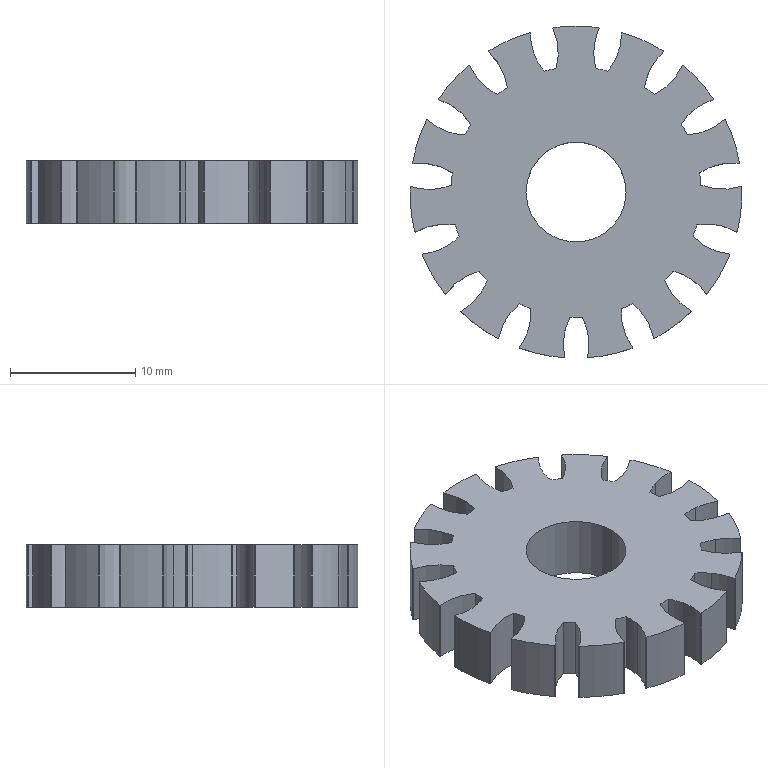Part | SolidWorks | features ICE 4, CirPattern 1, Extrusion 1 | 1 solid | 110 faces | box 26.541 x 26.503 x 5 mm | volume 2075 mm3 | cylinder 108 | plane 2 | commonest cylinder face diameters 9.371 x45 6.629 x30 26.541 x16 20 x15 8 x2